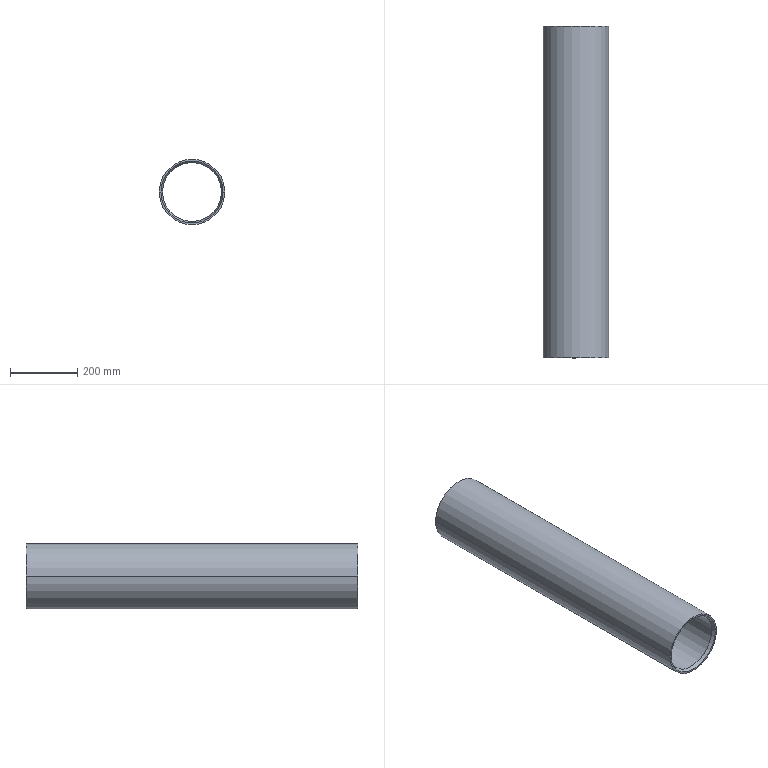Part | STEP file | Roller XG1 | 1 solid | 10 faces | box 195 x 987 x 195 mm | volume 5708379 mm3 | cone 4 | cylinder 4 | plane 2 | commonest cylinder face diameters 175 x2 195 x2
STEP:
#1=CARTESIAN_POINT('',(0.,0.,0.));
#2=DIRECTION('',(0.,0.,1.));
#3=DIRECTION('',(1.,0.,0.));
#4=AXIS2_PLACEMENT_3D('',#1,#2,#3);
#5=CARTESIAN_POINT('',(-87.5,483.5,0.));
#6=VERTEX_POINT('',#5);
#7=CARTESIAN_POINT('',(-92.5,493.5,0.));
#8=VERTEX_POINT('',#7);
#9=CARTESIAN_POINT('',(-92.5,493.5,0.));
#10=DIRECTION('',(-0.4472,0.8944,0.));
#11=VECTOR('',#10,1.);
#12=LINE('',#9,#11);
#13=CARTESIAN_POINT('',(0.,493.5,0.));
#14=DIRECTION('',(0.,1.,0.));
#15=DIRECTION('',(-1.,0.,0.));
#16=AXIS2_PLACEMENT_3D('',#13,#14,#15);
#17=CONICAL_SURFACE('',#16,92.5,0.4636);
#18=CARTESIAN_POINT('',(6.283,0.));
#19=DIRECTION('',(0.,1.));
#20=VECTOR('',#19,1.);
#21=LINE('',#18,#20);
#22=(GEOMETRIC_REPRESENTATION_CONTEXT(2)PARAMETRIC_REPRESENTATION_CONTEXT()REPRESENTATION_CONTEXT('',''));
#23=DEFINITIONAL_REPRESENTATION('',(#21),#22);
#24=PCURVE('',#17,#23);
#25=CARTESIAN_POINT('',(0.,493.5,0.));
#26=DIRECTION('',(0.,1.,0.));
#27=DIRECTION('',(-1.,0.,0.));
#28=AXIS2_PLACEMENT_3D('',#25,#26,#27);
#29=CONICAL_SURFACE('',#28,92.5,0.4636);
#30=CARTESIAN_POINT('',(0.,0.));
#31=DIRECTION('',(0.,1.));
#32=VECTOR('',#31,1.);
#33=LINE('',#30,#32);
#34=(GEOMETRIC_REPRESENTATION_CONTEXT(2)PARAMETRIC_REPRESENTATION_CONTEXT()REPRESENTATION_CONTEXT('',''));
#35=DEFINITIONAL_REPRESENTATION('',(#33),#34);
#36=PCURVE('',#29,#35);
#37=SURFACE_CURVE('',#12,(#24,#36),.PCURVE_S1.);
#38=EDGE_CURVE('',#6,#8,#37,.T.);
#39=ORIENTED_EDGE('',*,*,#38,.T.);
#40=CARTESIAN_POINT('',(92.5,493.5,0.));
#41=VERTEX_POINT('',#40);
#42=CARTESIAN_POINT('',(0.,493.5,0.));
#43=DIRECTION('',(0.,-1.,0.));
#44=DIRECTION('',(-1.,0.,0.));
#45=AXIS2_PLACEMENT_3D('',#42,#43,#44);
#46=CIRCLE('',#45,92.5);
#47=CARTESIAN_POINT('',(6.283,0.));
#48=DIRECTION('',(-1.,0.));
#49=VECTOR('',#48,1.);
#50=LINE('',#47,#49);
#51=(GEOMETRIC_REPRESENTATION_CONTEXT(2)PARAMETRIC_REPRESENTATION_CONTEXT()REPRESENTATION_CONTEXT('',''));
#52=DEFINITIONAL_REPRESENTATION('',(#50),#51);
#53=PCURVE('',#17,#52);
#54=CARTESIAN_POINT('',(87.5,493.5,0.));
#55=DIRECTION('',(0.,1.,0.));
#56=DIRECTION('',(-1.,0.,0.));
#57=AXIS2_PLACEMENT_3D('',#54,#55,#56);
#58=PLANE('',#57);
#59=CARTESIAN_POINT('',(180.,0.));
#60=CARTESIAN_POINT('',(180.,-160.215));
#61=CARTESIAN_POINT('',(41.25,-80.107));
#62=CARTESIAN_POINT('',(-97.5,0.));
#63=CARTESIAN_POINT('',(41.25,80.107));
#64=CARTESIAN_POINT('',(180.,160.215));
#65=CARTESIAN_POINT('',(180.,0.));
#66=(BOUNDED_CURVE()B_SPLINE_CURVE(2,(#59,#60,#61,#62,#63,#64,#65),.UNSPECIFIED.,.T.,.F.)B_SPLINE_CURVE_WITH_KNOTS((1,2,2,2,2,1),(-2.094,0.,2.094,4.189,6.283,8.378),.UNSPECIFIED.)CURVE()GEOMETRIC_REPRESENTATION_ITEM()RATIONAL_B_SPLINE_CURVE((1.,0.5,1.,0.5,1.,0.5,1.))REPRESENTATION_ITEM(''));
#67=(GEOMETRIC_REPRESENTATION_CONTEXT(2)PARAMETRIC_REPRESENTATION_CONTEXT()REPRESENTATION_CONTEXT('',''));
#68=DEFINITIONAL_REPRESENTATION('',(#66),#67);
#69=PCURVE('',#58,#68);
#70=SURFACE_CURVE('',#46,(#53,#69),.PCURVE_S1.);
#71=EDGE_CURVE('',#8,#41,#70,.T.);
#72=ORIENTED_EDGE('',*,*,#71,.T.);
#73=CARTESIAN_POINT('',(87.5,483.5,0.));
#74=VERTEX_POINT('',#73);
#75=CARTESIAN_POINT('',(92.5,493.5,0.));
#76=DIRECTION('',(0.4472,0.8944,0.));
#77=VECTOR('',#76,1.);
#78=LINE('',#75,#77);
#79=CARTESIAN_POINT('',(3.142,0.));
#80=DIRECTION('',(0.,1.));
#81=VECTOR('',#80,1.);
#82=LINE('',#79,#81);
#83=(GEOMETRIC_REPRESENTATION_CONTEXT(2)PARAMETRIC_REPRESENTATION_CONTEXT()REPRESENTATION_CONTEXT('',''));
#84=DEFINITIONAL_REPRESENTATION('',(#82),#83);
#85=PCURVE('',#17,#84);
#86=CARTESIAN_POINT('',(3.142,0.));
#87=DIRECTION('',(0.,1.));
#88=VECTOR('',#87,1.);
#89=LINE('',#86,#88);
#90=(GEOMETRIC_REPRESENTATION_CONTEXT(2)PARAMETRIC_REPRESENTATION_CONTEXT()REPRESENTATION_CONTEXT('',''));
#91=DEFINITIONAL_REPRESENTATION('',(#89),#90);
#92=PCURVE('',#29,#91);
#93=SURFACE_CURVE('',#78,(#85,#92),.PCURVE_S1.);
#94=EDGE_CURVE('',#74,#41,#93,.T.);
#95=ORIENTED_EDGE('',*,*,#94,.F.);
#96=CARTESIAN_POINT('',(0.,483.5,0.));
#97=DIRECTION('',(0.,1.,0.));
#98=DIRECTION('',(-1.,0.,0.));
#99=AXIS2_PLACEMENT_3D('',#96,#97,#98);
#100=CIRCLE('',#99,87.5);
#101=CARTESIAN_POINT('',(0.,-10.));
#102=DIRECTION('',(1.,0.));
#103=VECTOR('',#102,1.);
#104=LINE('',#101,#103);
#105=(GEOMETRIC_REPRESENTATION_CONTEXT(2)PARAMETRIC_REPRESENTATION_CONTEXT()REPRESENTATION_CONTEXT('',''));
#106=DEFINITIONAL_REPRESENTATION('',(#104),#105);
#107=PCURVE('',#17,#106);
#108=CARTESIAN_POINT('',(0.,-1054.436,0.));
#109=DIRECTION('',(0.,-1.,0.));
#110=DIRECTION('',(1.,0.,0.));
#111=AXIS2_PLACEMENT_3D('',#108,#109,#110);
#112=CYLINDRICAL_SURFACE('',#111,87.5);
#113=CARTESIAN_POINT('',(9.425,-1537.936));
#114=DIRECTION('',(-1.,0.));
#115=VECTOR('',#114,1.);
#116=LINE('',#113,#115);
#117=(GEOMETRIC_REPRESENTATION_CONTEXT(2)PARAMETRIC_REPRESENTATION_CONTEXT()REPRESENTATION_CONTEXT('',''));
#118=DEFINITIONAL_REPRESENTATION('',(#116),#117);
#119=PCURVE('',#112,#118);
#120=SURFACE_CURVE('',#100,(#107,#119),.PCURVE_S1.);
#121=EDGE_CURVE('',#74,#6,#120,.T.);
#122=ORIENTED_EDGE('',*,*,#121,.T.);
#123=EDGE_LOOP('',(#39,#72,#95,#122));
#124=FACE_BOUND('',#123,.F.);
#125=ADVANCED_FACE('',(#124),#17,.F.);
#126=CARTESIAN_POINT('',(87.5,-483.5,0.));
#127=VERTEX_POINT('',#126);
#128=CARTESIAN_POINT('',(92.5,-493.5,0.));
#129=VERTEX_POINT('',#128);
#130=CARTESIAN_POINT('',(87.5,-483.5,0.));
#131=DIRECTION('',(0.4472,-0.8944,0.));
#132=VECTOR('',#131,1.);
#133=LINE('',#130,#132);
#134=CARTESIAN_POINT('',(0.,-483.5,0.));
#135=DIRECTION('',(0.,-1.,0.));
#136=DIRECTION('',(1.,0.,0.));
#137=AXIS2_PLACEMENT_3D('',#134,#135,#136);
#138=CONICAL_SURFACE('',#137,87.5,0.4636);
#139=CARTESIAN_POINT('',(6.283,0.));
#140=DIRECTION('',(0.,1.));
#141=VECTOR('',#140,1.);
#142=LINE('',#139,#141);
#143=(GEOMETRIC_REPRESENTATION_CONTEXT(2)PARAMETRIC_REPRESENTATION_CONTEXT()REPRESENTATION_CONTEXT('',''));
#144=DEFINITIONAL_REPRESENTATION('',(#142),#143);
#145=PCURVE('',#138,#144);
#146=CARTESIAN_POINT('',(0.,-483.5,0.));
#147=DIRECTION('',(0.,-1.,0.));
#148=DIRECTION('',(1.,0.,0.));
#149=AXIS2_PLACEMENT_3D('',#146,#147,#148);
#150=CONICAL_SURFACE('',#149,87.5,0.4636);
#151=CARTESIAN_POINT('',(0.,0.));
#152=DIRECTION('',(0.,1.));
#153=VECTOR('',#152,1.);
#154=LINE('',#151,#153);
#155=(GEOMETRIC_REPRESENTATION_CONTEXT(2)PARAMETRIC_REPRESENTATION_CONTEXT()REPRESENTATION_CONTEXT('',''));
#156=DEFINITIONAL_REPRESENTATION('',(#154),#155);
#157=PCURVE('',#150,#156);
#158=SURFACE_CURVE('',#133,(#145,#157),.PCURVE_S1.);
#159=EDGE_CURVE('',#127,#129,#158,.T.);
#160=ORIENTED_EDGE('',*,*,#159,.T.);
#161=CARTESIAN_POINT('',(-92.5,-493.5,0.));
#162=VERTEX_POINT('',#161);
#163=CARTESIAN_POINT('',(0.,-493.5,0.));
#164=DIRECTION('',(0.,1.,0.));
#165=DIRECTION('',(1.,0.,0.));
#166=AXIS2_PLACEMENT_3D('',#163,#164,#165);
#167=CIRCLE('',#166,92.5);
#168=CARTESIAN_POINT('',(6.283,10.));
#169=DIRECTION('',(-1.,0.));
#170=VECTOR('',#169,1.);
#171=LINE('',#168,#170);
#172=(GEOMETRIC_REPRESENTATION_CONTEXT(2)PARAMETRIC_REPRESENTATION_CONTEXT()REPRESENTATION_CONTEXT('',''));
#173=DEFINITIONAL_REPRESENTATION('',(#171),#172);
#174=PCURVE('',#138,#173);
#175=CARTESIAN_POINT('',(87.5,-493.5,0.));
#176=DIRECTION('',(0.,-1.,0.));
#177=DIRECTION('',(1.,0.,0.));
#178=AXIS2_PLACEMENT_3D('',#175,#176,#177);
#179=PLANE('',#178);
#180=CARTESIAN_POINT('',(5.,0.));
#181=CARTESIAN_POINT('',(5.,-160.215));
#182=CARTESIAN_POINT('',(-133.75,-80.107));
#183=CARTESIAN_POINT('',(-272.5,0.));
#184=CARTESIAN_POINT('',(-133.75,80.107));
#185=CARTESIAN_POINT('',(5.,160.215));
#186=CARTESIAN_POINT('',(5.,0.));
#187=(BOUNDED_CURVE()B_SPLINE_CURVE(2,(#180,#181,#182,#183,#184,#185,#186),.UNSPECIFIED.,.T.,.F.)B_SPLINE_CURVE_WITH_KNOTS((1,2,2,2,2,1),(-2.094,0.,2.094,4.189,6.283,8.378),.UNSPECIFIED.)CURVE()GEOMETRIC_REPRESENTATION_ITEM()RATIONAL_B_SPLINE_CURVE((1.,0.5,1.,0.5,1.,0.5,1.))REPRESENTATION_ITEM(''));
#188=(GEOMETRIC_REPRESENTATION_CONTEXT(2)PARAMETRIC_REPRESENTATION_CONTEXT()REPRESENTATION_CONTEXT('',''));
#189=DEFINITIONAL_REPRESENTATION('',(#187),#188);
#190=PCURVE('',#179,#189);
#191=SURFACE_CURVE('',#167,(#174,#190),.PCURVE_S1.);
#192=EDGE_CURVE('',#129,#162,#191,.T.);
#193=ORIENTED_EDGE('',*,*,#192,.T.);
#194=CARTESIAN_POINT('',(-87.5,-483.5,0.));
#195=VERTEX_POINT('',#194);
#196=CARTESIAN_POINT('',(-87.5,-483.5,0.));
#197=DIRECTION('',(-0.4472,-0.8944,0.));
#198=VECTOR('',#197,1.);
#199=LINE('',#196,#198);
#200=CARTESIAN_POINT('',(3.142,0.));
#201=DIRECTION('',(0.,1.));
#202=VECTOR('',#201,1.);
#203=LINE('',#200,#202);
#204=(GEOMETRIC_REPRESENTATION_CONTEXT(2)PARAMETRIC_REPRESENTATION_CONTEXT()REPRESENTATION_CONTEXT('',''));
#205=DEFINITIONAL_REPRESENTATION('',(#203),#204);
#206=PCURVE('',#138,#205);
#207=CARTESIAN_POINT('',(3.142,0.));
#208=DIRECTION('',(0.,1.));
#209=VECTOR('',#208,1.);
#210=LINE('',#207,#209);
#211=(GEOMETRIC_REPRESENTATION_CONTEXT(2)PARAMETRIC_REPRESENTATION_CONTEXT()REPRESENTATION_CONTEXT('',''));
#212=DEFINITIONAL_REPRESENTATION('',(#210),#211);
#213=PCURVE('',#150,#212);
#214=SURFACE_CURVE('',#199,(#206,#213),.PCURVE_S1.);
#215=EDGE_CURVE('',#195,#162,#214,.T.);
#216=ORIENTED_EDGE('',*,*,#215,.F.);
#217=CARTESIAN_POINT('',(0.,-483.5,0.));
#218=DIRECTION('',(0.,-1.,0.));
#219=DIRECTION('',(1.,0.,0.));
#220=AXIS2_PLACEMENT_3D('',#217,#218,#219);
#221=CIRCLE('',#220,87.5);
#222=CARTESIAN_POINT('',(0.,0.));
#223=DIRECTION('',(1.,0.));
#224=VECTOR('',#223,1.);
#225=LINE('',#222,#224);
#226=(GEOMETRIC_REPRESENTATION_CONTEXT(2)PARAMETRIC_REPRESENTATION_CONTEXT()REPRESENTATION_CONTEXT('',''));
#227=DEFINITIONAL_REPRESENTATION('',(#225),#226);
#228=PCURVE('',#138,#227);
#229=CARTESIAN_POINT('',(0.,-570.936));
#230=DIRECTION('',(1.,0.));
#231=VECTOR('',#230,1.);
#232=LINE('',#229,#231);
#233=(GEOMETRIC_REPRESENTATION_CONTEXT(2)PARAMETRIC_REPRESENTATION_CONTEXT()REPRESENTATION_CONTEXT('',''));
#234=DEFINITIONAL_REPRESENTATION('',(#232),#233);
#235=PCURVE('',#112,#234);
#236=SURFACE_CURVE('',#221,(#228,#235),.PCURVE_S1.);
#237=EDGE_CURVE('',#195,#127,#236,.T.);
#238=ORIENTED_EDGE('',*,*,#237,.T.);
#239=EDGE_LOOP('',(#160,#193,#216,#238));
#240=FACE_BOUND('',#239,.F.);
#241=ADVANCED_FACE('',(#240),#138,.F.);
#242=CARTESIAN_POINT('',(97.5,493.5,0.));
#243=VERTEX_POINT('',#242);
#244=CARTESIAN_POINT('',(-97.5,493.5,0.));
#245=VERTEX_POINT('',#244);
#246=CARTESIAN_POINT('',(0.,493.5,0.));
#247=DIRECTION('',(0.,-1.,0.));
#248=DIRECTION('',(1.,0.,0.));
#249=AXIS2_PLACEMENT_3D('',#246,#247,#248);
#250=CIRCLE('',#249,97.5);
#251=CARTESIAN_POINT('',(0.,-1054.436,0.));
#252=DIRECTION('',(0.,-1.,0.));
#253=DIRECTION('',(1.,0.,0.));
#254=AXIS2_PLACEMENT_3D('',#251,#252,#253);
#255=CYLINDRICAL_SURFACE('',#254,97.5);
#256=CARTESIAN_POINT('',(0.,-1547.936));
#257=DIRECTION('',(1.,0.));
#258=VECTOR('',#257,1.);
#259=LINE('',#256,#258);
#260=(GEOMETRIC_REPRESENTATION_CONTEXT(2)PARAMETRIC_REPRESENTATION_CONTEXT()REPRESENTATION_CONTEXT('',''));
#261=DEFINITIONAL_REPRESENTATION('',(#259),#260);
#262=PCURVE('',#255,#261);
#263=CARTESIAN_POINT('',(-10.,0.));
#264=CARTESIAN_POINT('',(-10.,168.875));
#265=CARTESIAN_POINT('',(136.25,84.437));
#266=CARTESIAN_POINT('',(282.5,0.));
#267=CARTESIAN_POINT('',(136.25,-84.437));
#268=CARTESIAN_POINT('',(-10.,-168.875));
#269=CARTESIAN_POINT('',(-10.,0.));
#270=(BOUNDED_CURVE()B_SPLINE_CURVE(2,(#263,#264,#265,#266,#267,#268,#269),.UNSPECIFIED.,.T.,.F.)B_SPLINE_CURVE_WITH_KNOTS((1,2,2,2,2,1),(-2.094,0.,2.094,4.189,6.283,8.378),.UNSPECIFIED.)CURVE()GEOMETRIC_REPRESENTATION_ITEM()RATIONAL_B_SPLINE_CURVE((1.,0.5,1.,0.5,1.,0.5,1.))REPRESENTATION_ITEM(''));
#271=(GEOMETRIC_REPRESENTATION_CONTEXT(2)PARAMETRIC_REPRESENTATION_CONTEXT()REPRESENTATION_CONTEXT('',''));
#272=DEFINITIONAL_REPRESENTATION('',(#270),#271);
#273=PCURVE('',#58,#272);
#274=SURFACE_CURVE('',#250,(#262,#273),.PCURVE_S1.);
#275=EDGE_CURVE('',#243,#245,#274,.T.);
#276=ORIENTED_EDGE('',*,*,#275,.T.);
#277=CARTESIAN_POINT('',(-97.5,-493.5,0.));
#278=VERTEX_POINT('',#277);
#279=CARTESIAN_POINT('',(-97.5,-1054.436,0.));
#280=DIRECTION('',(0.,-1.,0.));
#281=VECTOR('',#280,1.);
#282=LINE('',#279,#281);
#283=CARTESIAN_POINT('',(3.142,0.));
#284=DIRECTION('',(0.,1.));
#285=VECTOR('',#284,1.);
#286=LINE('',#283,#285);
#287=(GEOMETRIC_REPRESENTATION_CONTEXT(2)PARAMETRIC_REPRESENTATION_CONTEXT()REPRESENTATION_CONTEXT('',''));
#288=DEFINITIONAL_REPRESENTATION('',(#286),#287);
#289=PCURVE('',#255,#288);
#290=CARTESIAN_POINT('',(0.,-1054.436,0.));
#291=DIRECTION('',(0.,-1.,0.));
#292=DIRECTION('',(1.,0.,0.));
#293=AXIS2_PLACEMENT_3D('',#290,#291,#292);
#294=CYLINDRICAL_SURFACE('',#293,97.5);
#295=CARTESIAN_POINT('',(3.142,0.));
#296=DIRECTION('',(0.,1.));
#297=VECTOR('',#296,1.);
#298=LINE('',#295,#297);
#299=(GEOMETRIC_REPRESENTATION_CONTEXT(2)PARAMETRIC_REPRESENTATION_CONTEXT()REPRESENTATION_CONTEXT('',''));
#300=DEFINITIONAL_REPRESENTATION('',(#298),#299);
#301=PCURVE('',#294,#300);
#302=SURFACE_CURVE('',#282,(#289,#301),.PCURVE_S1.);
#303=EDGE_CURVE('',#245,#278,#302,.T.);
#304=ORIENTED_EDGE('',*,*,#303,.T.);
#305=CARTESIAN_POINT('',(97.5,-493.5,0.));
#306=VERTEX_POINT('',#305);
#307=CARTESIAN_POINT('',(0.,-493.5,0.));
#308=DIRECTION('',(0.,-1.,0.));
#309=DIRECTION('',(1.,0.,0.));
#310=AXIS2_PLACEMENT_3D('',#307,#308,#309);
#311=CIRCLE('',#310,97.5);
#312=CARTESIAN_POINT('',(0.,-560.936));
#313=DIRECTION('',(1.,0.));
#314=VECTOR('',#313,1.);
#315=LINE('',#312,#314);
#316=(GEOMETRIC_REPRESENTATION_CONTEXT(2)PARAMETRIC_REPRESENTATION_CONTEXT()REPRESENTATION_CONTEXT('',''));
#317=DEFINITIONAL_REPRESENTATION('',(#315),#316);
#318=PCURVE('',#255,#317);
#319=CARTESIAN_POINT('',(-87.5,0.));
#320=DIRECTION('',(1.,0.));
#321=AXIS2_PLACEMENT_2D('',#319,#320);
#322=CIRCLE('',#321,97.5);
#323=(GEOMETRIC_REPRESENTATION_CONTEXT(2)PARAMETRIC_REPRESENTATION_CONTEXT()REPRESENTATION_CONTEXT('',''));
#324=DEFINITIONAL_REPRESENTATION('',(#322),#323);
#325=PCURVE('',#179,#324);
#326=SURFACE_CURVE('',#311,(#318,#325),.PCURVE_S1.);
#327=EDGE_CURVE('',#306,#278,#326,.T.);
#328=ORIENTED_EDGE('',*,*,#327,.F.);
#329=CARTESIAN_POINT('',(97.5,-1054.436,0.));
#330=DIRECTION('',(0.,-1.,0.));
#331=VECTOR('',#330,1.);
#332=LINE('',#329,#331);
#333=CARTESIAN_POINT('',(0.,0.));
#334=DIRECTION('',(0.,1.));
#335=VECTOR('',#334,1.);
#336=LINE('',#333,#335);
#337=(GEOMETRIC_REPRESENTATION_CONTEXT(2)PARAMETRIC_REPRESENTATION_CONTEXT()REPRESENTATION_CONTEXT('',''));
#338=DEFINITIONAL_REPRESENTATION('',(#336),#337);
#339=PCURVE('',#255,#338);
#340=CARTESIAN_POINT('',(6.283,0.));
#341=DIRECTION('',(0.,1.));
#342=VECTOR('',#341,1.);
#343=LINE('',#340,#342);
#344=(GEOMETRIC_REPRESENTATION_CONTEXT(2)PARAMETRIC_REPRESENTATION_CONTEXT()REPRESENTATION_CONTEXT('',''));
#345=DEFINITIONAL_REPRESENTATION('',(#343),#344);
#346=PCURVE('',#294,#345);
#347=SURFACE_CURVE('',#332,(#339,#346),.PCURVE_S1.);
#348=EDGE_CURVE('',#243,#306,#347,.T.);
#349=ORIENTED_EDGE('',*,*,#348,.F.);
#350=EDGE_LOOP('',(#276,#304,#328,#349));
#351=FACE_BOUND('',#350,.T.);
#352=ADVANCED_FACE('',(#351),#255,.T.);
#353=CARTESIAN_POINT('',(87.5,-1054.436,0.));
#354=DIRECTION('',(0.,-1.,0.));
#355=VECTOR('',#354,1.);
#356=LINE('',#353,#355);
#357=CARTESIAN_POINT('',(6.283,0.));
#358=DIRECTION('',(0.,1.));
#359=VECTOR('',#358,1.);
#360=LINE('',#357,#359);
#361=(GEOMETRIC_REPRESENTATION_CONTEXT(2)PARAMETRIC_REPRESENTATION_CONTEXT()REPRESENTATION_CONTEXT('',''));
#362=DEFINITIONAL_REPRESENTATION('',(#360),#361);
#363=PCURVE('',#112,#362);
#364=CARTESIAN_POINT('',(0.,-1054.436,0.));
#365=DIRECTION('',(0.,-1.,0.));
#366=DIRECTION('',(1.,0.,0.));
#367=AXIS2_PLACEMENT_3D('',#364,#365,#366);
#368=CYLINDRICAL_SURFACE('',#367,87.5);
#369=CARTESIAN_POINT('',(0.,0.));
#370=DIRECTION('',(0.,1.));
#371=VECTOR('',#370,1.);
#372=LINE('',#369,#371);
#373=(GEOMETRIC_REPRESENTATION_CONTEXT(2)PARAMETRIC_REPRESENTATION_CONTEXT()REPRESENTATION_CONTEXT('',''));
#374=DEFINITIONAL_REPRESENTATION('',(#372),#373);
#375=PCURVE('',#368,#374);
#376=SURFACE_CURVE('',#356,(#363,#375),.PCURVE_S1.);
#377=EDGE_CURVE('',#74,#127,#376,.T.);
#378=ORIENTED_EDGE('',*,*,#377,.T.);
#379=ORIENTED_EDGE('',*,*,#237,.F.);
#380=CARTESIAN_POINT('',(-87.5,-1054.436,0.));
#381=DIRECTION('',(0.,-1.,0.));
#382=VECTOR('',#381,1.);
#383=LINE('',#380,#382);
#384=CARTESIAN_POINT('',(3.142,0.));
#385=DIRECTION('',(0.,1.));
#386=VECTOR('',#385,1.);
#387=LINE('',#384,#386);
#388=(GEOMETRIC_REPRESENTATION_CONTEXT(2)PARAMETRIC_REPRESENTATION_CONTEXT()REPRESENTATION_CONTEXT('',''));
#389=DEFINITIONAL_REPRESENTATION('',(#387),#388);
#390=PCURVE('',#112,#389);
#391=CARTESIAN_POINT('',(3.142,0.));
#392=DIRECTION('',(0.,1.));
#393=VECTOR('',#392,1.);
#394=LINE('',#391,#393);
#395=(GEOMETRIC_REPRESENTATION_CONTEXT(2)PARAMETRIC_REPRESENTATION_CONTEXT()REPRESENTATION_CONTEXT('',''));
#396=DEFINITIONAL_REPRESENTATION('',(#394),#395);
#397=PCURVE('',#368,#396);
#398=SURFACE_CURVE('',#383,(#390,#397),.PCURVE_S1.);
#399=EDGE_CURVE('',#6,#195,#398,.T.);
#400=ORIENTED_EDGE('',*,*,#399,.F.);
#401=ORIENTED_EDGE('',*,*,#121,.F.);
#402=EDGE_LOOP('',(#378,#379,#400,#401));
#403=FACE_BOUND('',#402,.F.);
#404=ADVANCED_FACE('',(#403),#112,.F.);
#405=CARTESIAN_POINT('',(0.,-483.5,0.));
#406=DIRECTION('',(0.,-1.,0.));
#407=DIRECTION('',(1.,0.,0.));
#408=AXIS2_PLACEMENT_3D('',#405,#406,#407);
#409=CIRCLE('',#408,87.5);
#410=CARTESIAN_POINT('',(0.,-570.936));
#411=DIRECTION('',(1.,0.));
#412=VECTOR('',#411,1.);
#413=LINE('',#410,#412);
#414=(GEOMETRIC_REPRESENTATION_CONTEXT(2)PARAMETRIC_REPRESENTATION_CONTEXT()REPRESENTATION_CONTEXT('',''));
#415=DEFINITIONAL_REPRESENTATION('',(#413),#414);
#416=PCURVE('',#368,#415);
#417=CARTESIAN_POINT('',(0.,0.));
#418=DIRECTION('',(1.,0.));
#419=VECTOR('',#418,1.);
#420=LINE('',#417,#419);
#421=(GEOMETRIC_REPRESENTATION_CONTEXT(2)PARAMETRIC_REPRESENTATION_CONTEXT()REPRESENTATION_CONTEXT('',''));
#422=DEFINITIONAL_REPRESENTATION('',(#420),#421);
#423=PCURVE('',#150,#422);
#424=SURFACE_CURVE('',#409,(#416,#423),.PCURVE_S1.);
#425=EDGE_CURVE('',#127,#195,#424,.T.);
#426=ORIENTED_EDGE('',*,*,#425,.F.);
#427=ORIENTED_EDGE('',*,*,#377,.F.);
#428=CARTESIAN_POINT('',(0.,483.5,0.));
#429=DIRECTION('',(0.,1.,0.));
#430=DIRECTION('',(-1.,0.,0.));
#431=AXIS2_PLACEMENT_3D('',#428,#429,#430);
#432=CIRCLE('',#431,87.5);
#433=CARTESIAN_POINT('',(3.142,-1537.936));
#434=DIRECTION('',(-1.,0.));
#435=VECTOR('',#434,1.);
#436=LINE('',#433,#435);
#437=(GEOMETRIC_REPRESENTATION_CONTEXT(2)PARAMETRIC_REPRESENTATION_CONTEXT()REPRESENTATION_CONTEXT('',''));
#438=DEFINITIONAL_REPRESENTATION('',(#436),#437);
#439=PCURVE('',#368,#438);
#440=CARTESIAN_POINT('',(0.,-10.));
#441=DIRECTION('',(1.,0.));
#442=VECTOR('',#441,1.);
#443=LINE('',#440,#442);
#444=(GEOMETRIC_REPRESENTATION_CONTEXT(2)PARAMETRIC_REPRESENTATION_CONTEXT()REPRESENTATION_CONTEXT('',''));
#445=DEFINITIONAL_REPRESENTATION('',(#443),#444);
#446=PCURVE('',#29,#445);
#447=SURFACE_CURVE('',#432,(#439,#446),.PCURVE_S1.);
#448=EDGE_CURVE('',#6,#74,#447,.T.);
#449=ORIENTED_EDGE('',*,*,#448,.F.);
#450=ORIENTED_EDGE('',*,*,#399,.T.);
#451=EDGE_LOOP('',(#426,#427,#449,#450));
#452=FACE_BOUND('',#451,.F.);
#453=ADVANCED_FACE('',(#452),#368,.F.);
#454=ORIENTED_EDGE('',*,*,#71,.T.);
#455=CARTESIAN_POINT('',(0.,493.5,0.));
#456=DIRECTION('',(0.,-1.,0.));
#457=DIRECTION('',(-1.,0.,0.));
#458=AXIS2_PLACEMENT_3D('',#455,#456,#457);
#459=CIRCLE('',#458,92.5);
#460=CARTESIAN_POINT('',(180.,0.));
#461=CARTESIAN_POINT('',(180.,-160.215));
#462=CARTESIAN_POINT('',(41.25,-80.107));
#463=CARTESIAN_POINT('',(-97.5,0.));
#464=CARTESIAN_POINT('',(41.25,80.107));
#465=CARTESIAN_POINT('',(180.,160.215));
#466=CARTESIAN_POINT('',(180.,0.));
#467=(BOUNDED_CURVE()B_SPLINE_CURVE(2,(#460,#461,#462,#463,#464,#465,#466),.UNSPECIFIED.,.T.,.F.)B_SPLINE_CURVE_WITH_KNOTS((1,2,2,2,2,1),(-2.094,0.,2.094,4.189,6.283,8.378),.UNSPECIFIED.)CURVE()GEOMETRIC_REPRESENTATION_ITEM()RATIONAL_B_SPLINE_CURVE((1.,0.5,1.,0.5,1.,0.5,1.))REPRESENTATION_ITEM(''));
#468=(GEOMETRIC_REPRESENTATION_CONTEXT(2)PARAMETRIC_REPRESENTATION_CONTEXT()REPRESENTATION_CONTEXT('',''));
#469=DEFINITIONAL_REPRESENTATION('',(#467),#468);
#470=PCURVE('',#58,#469);
#471=CARTESIAN_POINT('',(6.283,0.));
#472=DIRECTION('',(-1.,0.));
#473=VECTOR('',#472,1.);
#474=LINE('',#471,#473);
#475=(GEOMETRIC_REPRESENTATION_CONTEXT(2)PARAMETRIC_REPRESENTATION_CONTEXT()REPRESENTATION_CONTEXT('',''));
#476=DEFINITIONAL_REPRESENTATION('',(#474),#475);
#477=PCURVE('',#29,#476);
#478=SURFACE_CURVE('',#459,(#470,#477),.PCURVE_S1.);
#479=EDGE_CURVE('',#41,#8,#478,.T.);
#480=ORIENTED_EDGE('',*,*,#479,.T.);
#481=EDGE_LOOP('',(#454,#480));
#482=FACE_BOUND('',#481,.T.);
#483=ORIENTED_EDGE('',*,*,#275,.F.);
#484=CARTESIAN_POINT('',(0.,493.5,0.));
#485=DIRECTION('',(0.,-1.,0.));
#486=DIRECTION('',(1.,0.,0.));
#487=AXIS2_PLACEMENT_3D('',#484,#485,#486);
#488=CIRCLE('',#487,97.5);
#489=CARTESIAN_POINT('',(-10.,0.));
#490=CARTESIAN_POINT('',(-10.,168.875));
#491=CARTESIAN_POINT('',(136.25,84.437));
#492=CARTESIAN_POINT('',(282.5,0.));
#493=CARTESIAN_POINT('',(136.25,-84.437));
#494=CARTESIAN_POINT('',(-10.,-168.875));
#495=CARTESIAN_POINT('',(-10.,0.));
#496=(BOUNDED_CURVE()B_SPLINE_CURVE(2,(#489,#490,#491,#492,#493,#494,#495),.UNSPECIFIED.,.T.,.F.)B_SPLINE_CURVE_WITH_KNOTS((1,2,2,2,2,1),(-2.094,0.,2.094,4.189,6.283,8.378),.UNSPECIFIED.)CURVE()GEOMETRIC_REPRESENTATION_ITEM()RATIONAL_B_SPLINE_CURVE((1.,0.5,1.,0.5,1.,0.5,1.))REPRESENTATION_ITEM(''));
#497=(GEOMETRIC_REPRESENTATION_CONTEXT(2)PARAMETRIC_REPRESENTATION_CONTEXT()REPRESENTATION_CONTEXT('',''));
#498=DEFINITIONAL_REPRESENTATION('',(#496),#497);
#499=PCURVE('',#58,#498);
#500=CARTESIAN_POINT('',(0.,-1547.936));
#501=DIRECTION('',(1.,0.));
#502=VECTOR('',#501,1.);
#503=LINE('',#500,#502);
#504=(GEOMETRIC_REPRESENTATION_CONTEXT(2)PARAMETRIC_REPRESENTATION_CONTEXT()REPRESENTATION_CONTEXT('',''));
#505=DEFINITIONAL_REPRESENTATION('',(#503),#504);
#506=PCURVE('',#294,#505);
#507=SURFACE_CURVE('',#488,(#499,#506),.PCURVE_S1.);
#508=EDGE_CURVE('',#245,#243,#507,.T.);
#509=ORIENTED_EDGE('',*,*,#508,.F.);
#510=EDGE_LOOP('',(#483,#509));
#511=FACE_BOUND('',#510,.T.);
#512=ADVANCED_FACE('',(#482,#511),#58,.T.);
#513=ORIENTED_EDGE('',*,*,#303,.F.);
#514=ORIENTED_EDGE('',*,*,#508,.T.);
#515=ORIENTED_EDGE('',*,*,#348,.T.);
#516=CARTESIAN_POINT('',(0.,-493.5,0.));
#517=DIRECTION('',(0.,-1.,0.));
#518=DIRECTION('',(1.,0.,0.));
#519=AXIS2_PLACEMENT_3D('',#516,#517,#518);
#520=CIRCLE('',#519,97.5);
#521=CARTESIAN_POINT('',(0.,-560.936));
#522=DIRECTION('',(1.,0.));
#523=VECTOR('',#522,1.);
#524=LINE('',#521,#523);
#525=(GEOMETRIC_REPRESENTATION_CONTEXT(2)PARAMETRIC_REPRESENTATION_CONTEXT()REPRESENTATION_CONTEXT('',''));
#526=DEFINITIONAL_REPRESENTATION('',(#524),#525);
#527=PCURVE('',#294,#526);
#528=CARTESIAN_POINT('',(-87.5,0.));
#529=DIRECTION('',(1.,0.));
#530=AXIS2_PLACEMENT_2D('',#528,#529);
#531=CIRCLE('',#530,97.5);
#532=(GEOMETRIC_REPRESENTATION_CONTEXT(2)PARAMETRIC_REPRESENTATION_CONTEXT()REPRESENTATION_CONTEXT('',''));
#533=DEFINITIONAL_REPRESENTATION('',(#531),#532);
#534=PCURVE('',#179,#533);
#535=SURFACE_CURVE('',#520,(#527,#534),.PCURVE_S1.);
#536=EDGE_CURVE('',#278,#306,#535,.T.);
#537=ORIENTED_EDGE('',*,*,#536,.F.);
#538=EDGE_LOOP('',(#513,#514,#515,#537));
#539=FACE_BOUND('',#538,.T.);
#540=ADVANCED_FACE('',(#539),#294,.T.);
#541=ORIENTED_EDGE('',*,*,#192,.T.);
#542=CARTESIAN_POINT('',(0.,-493.5,0.));
#543=DIRECTION('',(0.,1.,0.));
#544=DIRECTION('',(1.,0.,0.));
#545=AXIS2_PLACEMENT_3D('',#542,#543,#544);
#546=CIRCLE('',#545,92.5);
#547=CARTESIAN_POINT('',(5.,0.));
#548=CARTESIAN_POINT('',(5.,-160.215));
#549=CARTESIAN_POINT('',(-133.75,-80.107));
#550=CARTESIAN_POINT('',(-272.5,0.));
#551=CARTESIAN_POINT('',(-133.75,80.107));
#552=CARTESIAN_POINT('',(5.,160.215));
#553=CARTESIAN_POINT('',(5.,0.));
#554=(BOUNDED_CURVE()B_SPLINE_CURVE(2,(#547,#548,#549,#550,#551,#552,#553),.UNSPECIFIED.,.T.,.F.)B_SPLINE_CURVE_WITH_KNOTS((1,2,2,2,2,1),(-2.094,0.,2.094,4.189,6.283,8.378),.UNSPECIFIED.)CURVE()GEOMETRIC_REPRESENTATION_ITEM()RATIONAL_B_SPLINE_CURVE((1.,0.5,1.,0.5,1.,0.5,1.))REPRESENTATION_ITEM(''));
#555=(GEOMETRIC_REPRESENTATION_CONTEXT(2)PARAMETRIC_REPRESENTATION_CONTEXT()REPRESENTATION_CONTEXT('',''));
#556=DEFINITIONAL_REPRESENTATION('',(#554),#555);
#557=PCURVE('',#179,#556);
#558=CARTESIAN_POINT('',(6.283,10.));
#559=DIRECTION('',(-1.,0.));
#560=VECTOR('',#559,1.);
#561=LINE('',#558,#560);
#562=(GEOMETRIC_REPRESENTATION_CONTEXT(2)PARAMETRIC_REPRESENTATION_CONTEXT()REPRESENTATION_CONTEXT('',''));
#563=DEFINITIONAL_REPRESENTATION('',(#561),#562);
#564=PCURVE('',#150,#563);
#565=SURFACE_CURVE('',#546,(#557,#564),.PCURVE_S1.);
#566=EDGE_CURVE('',#162,#129,#565,.T.);
#567=ORIENTED_EDGE('',*,*,#566,.T.);
#568=EDGE_LOOP('',(#541,#567));
#569=FACE_BOUND('',#568,.T.);
#570=ORIENTED_EDGE('',*,*,#327,.T.);
#571=ORIENTED_EDGE('',*,*,#536,.T.);
#572=EDGE_LOOP('',(#570,#571));
#573=FACE_BOUND('',#572,.T.);
#574=ADVANCED_FACE('',(#569,#573),#179,.T.);
#575=ORIENTED_EDGE('',*,*,#566,.T.);
#576=ORIENTED_EDGE('',*,*,#159,.F.);
#577=ORIENTED_EDGE('',*,*,#425,.T.);
#578=ORIENTED_EDGE('',*,*,#215,.T.);
#579=EDGE_LOOP('',(#575,#576,#577,#578));
#580=FACE_BOUND('',#579,.F.);
#581=ADVANCED_FACE('',(#580),#150,.F.);
#582=ORIENTED_EDGE('',*,*,#479,.T.);
#583=ORIENTED_EDGE('',*,*,#38,.F.);
#584=ORIENTED_EDGE('',*,*,#448,.T.);
#585=ORIENTED_EDGE('',*,*,#94,.T.);
#586=EDGE_LOOP('',(#582,#583,#584,#585));
#587=FACE_BOUND('',#586,.F.);
#588=ADVANCED_FACE('',(#587),#29,.F.);
#589=CLOSED_SHELL('',(#125,#241,#352,#404,#453,#512,#540,#574,#581,#588));
#590=MANIFOLD_SOLID_BREP('',#589);
#591=(LENGTH_UNIT()NAMED_UNIT(*)SI_UNIT(.MILLI.,.METRE.));
#592=UNCERTAINTY_MEASURE_WITH_UNIT(LENGTH_MEASURE(0.0000001),#591,'','');
#593=(NAMED_UNIT(*)PLANE_ANGLE_UNIT()SI_UNIT($,.RADIAN.));
#594=(NAMED_UNIT(*)SI_UNIT($,.STERADIAN.)SOLID_ANGLE_UNIT());
#595=(GEOMETRIC_REPRESENTATION_CONTEXT(3)GLOBAL_UNCERTAINTY_ASSIGNED_CONTEXT((#592))GLOBAL_UNIT_ASSIGNED_CONTEXT((#591,#593,#594))REPRESENTATION_CONTEXT('',''));
#596=ADVANCED_BREP_SHAPE_REPRESENTATION('',(#4,#590),#595);